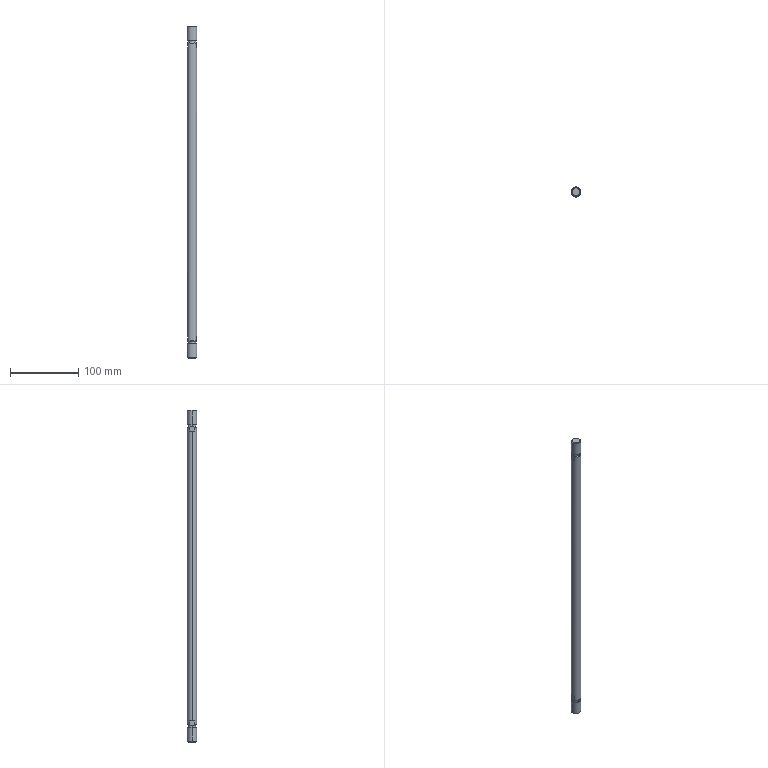Part | STEP file | rod_A_CDM2WB40_150_C76_0_ | 1 solid | 30 faces | box 14 x 14 x 488 mm | volume 74574 mm3 | plane 12 | cylinder 10 | cone 8 | commonest cylinder face diameters 14 x6 11.55 x4
STEP:
#1=CARTESIAN_POINT('',(5.775,0.,-454.));
#2=VERTEX_POINT('',#1);
#3=CARTESIAN_POINT('',(-5.775,0.,-454.));
#4=VERTEX_POINT('',#3);
#5=CARTESIAN_POINT('',(0.,0.,-454.));
#6=DIRECTION('',(0.,0.,1.));
#7=DIRECTION('',(1.,0.,0.));
#8=AXIS2_PLACEMENT_3D('',#5,#6,#7);
#9=CIRCLE('',#8,5.775);
#10=EDGE_CURVE('',#2,#4,#9,.T.);
#11=ORIENTED_EDGE('',*,*,#10,.T.);
#12=CARTESIAN_POINT('',(-7.,0.,-452.775));
#13=VERTEX_POINT('',#12);
#14=CARTESIAN_POINT('',(-5.775,0.,-454.));
#15=DIRECTION('',(-0.7071,0.,0.7071));
#16=VECTOR('',#15,1000.);
#17=LINE('',#14,#16);
#18=EDGE_CURVE('',#4,#13,#17,.T.);
#19=ORIENTED_EDGE('',*,*,#18,.T.);
#20=CARTESIAN_POINT('',(7.,0.,-452.775));
#21=VERTEX_POINT('',#20);
#22=CARTESIAN_POINT('',(0.,0.,-452.775));
#23=DIRECTION('',(0.,0.,1.));
#24=DIRECTION('',(1.,0.,0.));
#25=AXIS2_PLACEMENT_3D('',#22,#23,#24);
#26=CIRCLE('',#25,7.);
#27=EDGE_CURVE('',#21,#13,#26,.T.);
#28=ORIENTED_EDGE('',*,*,#27,.F.);
#29=CARTESIAN_POINT('',(5.775,0.,-454.));
#30=DIRECTION('',(0.7071,0.,0.7071));
#31=VECTOR('',#30,1000.);
#32=LINE('',#29,#31);
#33=EDGE_CURVE('',#2,#21,#32,.T.);
#34=ORIENTED_EDGE('',*,*,#33,.F.);
#35=EDGE_LOOP('',(#11,#19,#28,#34));
#36=FACE_OUTER_BOUND('',#35,.T.);
#37=CARTESIAN_POINT('',(0.,0.,-454.));
#38=DIRECTION('',(0.,0.,1.));
#39=DIRECTION('',(1.,0.,0.));
#40=AXIS2_PLACEMENT_3D('',#37,#38,#39);
#41=CONICAL_SURFACE('',#40,5.775,0.7854);
#42=ADVANCED_FACE('',(#36),#41,.T.);
#43=ORIENTED_EDGE('',*,*,#27,.T.);
#44=CARTESIAN_POINT('',(-7.,0.,-433.));
#45=VERTEX_POINT('',#44);
#46=CARTESIAN_POINT('',(-7.,0.,-454.));
#47=DIRECTION('',(0.,0.,1.));
#48=VECTOR('',#47,1000.);
#49=LINE('',#46,#48);
#50=EDGE_CURVE('',#13,#45,#49,.T.);
#51=ORIENTED_EDGE('',*,*,#50,.T.);
#52=CARTESIAN_POINT('',(7.,0.,-433.));
#53=VERTEX_POINT('',#52);
#54=CARTESIAN_POINT('',(0.,0.,-433.));
#55=DIRECTION('',(0.,0.,1.));
#56=DIRECTION('',(1.,0.,0.));
#57=AXIS2_PLACEMENT_3D('',#54,#55,#56);
#58=CIRCLE('',#57,7.);
#59=EDGE_CURVE('',#53,#45,#58,.T.);
#60=ORIENTED_EDGE('',*,*,#59,.F.);
#61=CARTESIAN_POINT('',(7.,0.,-454.));
#62=DIRECTION('',(0.,0.,1.));
#63=VECTOR('',#62,1000.);
#64=LINE('',#61,#63);
#65=EDGE_CURVE('',#21,#53,#64,.T.);
#66=ORIENTED_EDGE('',*,*,#65,.F.);
#67=EDGE_LOOP('',(#43,#51,#60,#66));
#68=FACE_OUTER_BOUND('',#67,.T.);
#69=CARTESIAN_POINT('',(0.,0.,-454.));
#70=DIRECTION('',(0.,0.,1.));
#71=DIRECTION('',(1.,0.,0.));
#72=AXIS2_PLACEMENT_3D('',#69,#70,#71);
#73=CYLINDRICAL_SURFACE('',#72,7.);
#74=ADVANCED_FACE('',(#68),#73,.T.);
#75=CARTESIAN_POINT('',(5.775,0.,-433.));
#76=VERTEX_POINT('',#75);
#77=CARTESIAN_POINT('',(-5.775,0.,-433.));
#78=VERTEX_POINT('',#77);
#79=CARTESIAN_POINT('',(0.,0.,-433.));
#80=DIRECTION('',(0.,0.,1.));
#81=DIRECTION('',(1.,0.,0.));
#82=AXIS2_PLACEMENT_3D('',#79,#80,#81);
#83=CIRCLE('',#82,5.775);
#84=EDGE_CURVE('',#76,#78,#83,.T.);
#85=ORIENTED_EDGE('',*,*,#84,.T.);
#86=CARTESIAN_POINT('',(-5.775,0.,-430.));
#87=VERTEX_POINT('',#86);
#88=CARTESIAN_POINT('',(-5.775,0.,-454.));
#89=DIRECTION('',(0.,0.,1.));
#90=VECTOR('',#89,1000.);
#91=LINE('',#88,#90);
#92=EDGE_CURVE('',#78,#87,#91,.T.);
#93=ORIENTED_EDGE('',*,*,#92,.T.);
#94=CARTESIAN_POINT('',(5.775,0.,-430.));
#95=VERTEX_POINT('',#94);
#96=CARTESIAN_POINT('',(0.,0.,-430.));
#97=DIRECTION('',(0.,0.,1.));
#98=DIRECTION('',(1.,0.,0.));
#99=AXIS2_PLACEMENT_3D('',#96,#97,#98);
#100=CIRCLE('',#99,5.775);
#101=EDGE_CURVE('',#95,#87,#100,.T.);
#102=ORIENTED_EDGE('',*,*,#101,.F.);
#103=CARTESIAN_POINT('',(5.775,0.,-454.));
#104=DIRECTION('',(0.,0.,1.));
#105=VECTOR('',#104,1000.);
#106=LINE('',#103,#105);
#107=EDGE_CURVE('',#76,#95,#106,.T.);
#108=ORIENTED_EDGE('',*,*,#107,.F.);
#109=EDGE_LOOP('',(#85,#93,#102,#108));
#110=FACE_OUTER_BOUND('',#109,.T.);
#111=CARTESIAN_POINT('',(0.,0.,-454.));
#112=DIRECTION('',(0.,0.,1.));
#113=DIRECTION('',(1.,0.,0.));
#114=AXIS2_PLACEMENT_3D('',#111,#112,#113);
#115=CYLINDRICAL_SURFACE('',#114,5.775);
#116=ADVANCED_FACE('',(#110),#115,.T.);
#117=ORIENTED_EDGE('',*,*,#101,.T.);
#118=CARTESIAN_POINT('',(-6.,0.,-429.775));
#119=VERTEX_POINT('',#118);
#120=CARTESIAN_POINT('',(-5.775,0.,-430.));
#121=DIRECTION('',(-0.7071,0.,0.7071));
#122=VECTOR('',#121,1000.);
#123=LINE('',#120,#122);
#124=EDGE_CURVE('',#87,#119,#123,.T.);
#125=ORIENTED_EDGE('',*,*,#124,.T.);
#126=CARTESIAN_POINT('',(-6.,3.606,-428.775));
#127=VERTEX_POINT('',#126);
#128=CARTESIAN_POINT('',(-6.,0.,-429.775));
#129=CARTESIAN_POINT('',(-6.,0.3144,-429.775));
#130=CARTESIAN_POINT('',(-6.,0.6332,-429.75));
#131=CARTESIAN_POINT('',(-6.,1.255,-429.653));
#132=CARTESIAN_POINT('',(-6.,1.561,-429.582));
#133=CARTESIAN_POINT('',(-6.,2.164,-429.403));
#134=CARTESIAN_POINT('',(-6.,2.462,-429.295));
#135=CARTESIAN_POINT('',(-6.,3.044,-429.052));
#136=CARTESIAN_POINT('',(-6.,3.328,-428.918));
#137=CARTESIAN_POINT('',(-6.,3.606,-428.775));
#138=B_SPLINE_CURVE_WITH_KNOTS('',3,(#128,#129,#130,#131,#132,#133,#134,#135,#136,#137),.UNSPECIFIED.,.F.,.F.,(4,2,2,2,4),(0.01366,0.0146,0.01554,0.01648,0.01742),.UNSPECIFIED.);
#139=EDGE_CURVE('',#119,#127,#138,.T.);
#140=ORIENTED_EDGE('',*,*,#139,.T.);
#141=CARTESIAN_POINT('',(6.,3.606,-428.775));
#142=VERTEX_POINT('',#141);
#143=CARTESIAN_POINT('',(0.,0.,-428.775));
#144=DIRECTION('',(0.,0.,1.));
#145=DIRECTION('',(1.,0.,0.));
#146=AXIS2_PLACEMENT_3D('',#143,#144,#145);
#147=CIRCLE('',#146,7.);
#148=EDGE_CURVE('',#142,#127,#147,.T.);
#149=ORIENTED_EDGE('',*,*,#148,.F.);
#150=CARTESIAN_POINT('',(6.,0.,-429.775));
#151=VERTEX_POINT('',#150);
#152=CARTESIAN_POINT('',(6.,3.606,-428.775));
#153=CARTESIAN_POINT('',(6.,3.328,-428.918));
#154=CARTESIAN_POINT('',(6.,3.044,-429.052));
#155=CARTESIAN_POINT('',(6.,2.462,-429.295));
#156=CARTESIAN_POINT('',(6.,2.164,-429.403));
#157=CARTESIAN_POINT('',(6.,1.561,-429.582));
#158=CARTESIAN_POINT('',(6.,1.255,-429.653));
#159=CARTESIAN_POINT('',(6.,0.6332,-429.75));
#160=CARTESIAN_POINT('',(6.,0.3144,-429.775));
#161=CARTESIAN_POINT('',(6.,0.,-429.775));
#162=B_SPLINE_CURVE_WITH_KNOTS('',3,(#152,#153,#154,#155,#156,#157,#158,#159,#160,#161),.UNSPECIFIED.,.F.,.F.,(4,2,2,2,4),(0.004778,0.005712,0.006646,0.00758,0.008514),.UNSPECIFIED.);
#163=EDGE_CURVE('',#142,#151,#162,.T.);
#164=ORIENTED_EDGE('',*,*,#163,.T.);
#165=CARTESIAN_POINT('',(5.775,0.,-430.));
#166=DIRECTION('',(0.7071,0.,0.7071));
#167=VECTOR('',#166,1000.);
#168=LINE('',#165,#167);
#169=EDGE_CURVE('',#95,#151,#168,.T.);
#170=ORIENTED_EDGE('',*,*,#169,.F.);
#171=EDGE_LOOP('',(#117,#125,#140,#149,#164,#170));
#172=FACE_OUTER_BOUND('',#171,.T.);
#173=CARTESIAN_POINT('',(0.,0.,-430.));
#174=DIRECTION('',(0.,0.,1.));
#175=DIRECTION('',(1.,0.,0.));
#176=AXIS2_PLACEMENT_3D('',#173,#174,#175);
#177=CONICAL_SURFACE('',#176,5.775,0.7854);
#178=ADVANCED_FACE('',(#172),#177,.T.);
#179=CARTESIAN_POINT('',(-6.,3.606,-423.));
#180=VERTEX_POINT('',#179);
#181=CARTESIAN_POINT('',(-7.,0.,-422.));
#182=VERTEX_POINT('',#181);
#183=CARTESIAN_POINT('',(-6.,3.606,-423.));
#184=CARTESIAN_POINT('',(-6.658,2.51,-422.342));
#185=CARTESIAN_POINT('',(-7.,1.278,-422.));
#186=CARTESIAN_POINT('',(-7.,0.,-422.));
#187=(BOUNDED_CURVE()B_SPLINE_CURVE(3,(#183,#184,#185,#186),.UNSPECIFIED.,.F.,.T.)B_SPLINE_CURVE_WITH_KNOTS((4,4),(5.742,6.283),.UNSPECIFIED.)CURVE()GEOMETRIC_REPRESENTATION_ITEM()RATIONAL_B_SPLINE_CURVE((1.,0.9757,0.9757,1.))REPRESENTATION_ITEM(''));
#188=EDGE_CURVE('',#180,#182,#187,.T.);
#189=ORIENTED_EDGE('',*,*,#188,.T.);
#190=CARTESIAN_POINT('',(-7.,0.,2.));
#191=VERTEX_POINT('',#190);
#192=CARTESIAN_POINT('',(-7.,0.,-454.));
#193=DIRECTION('',(0.,0.,1.));
#194=VECTOR('',#193,1000.);
#195=LINE('',#192,#194);
#196=EDGE_CURVE('',#182,#191,#195,.T.);
#197=ORIENTED_EDGE('',*,*,#196,.T.);
#198=CARTESIAN_POINT('',(-6.,3.606,3.));
#199=VERTEX_POINT('',#198);
#200=CARTESIAN_POINT('',(-7.,0.,2.));
#201=CARTESIAN_POINT('',(-7.,1.278,2.));
#202=CARTESIAN_POINT('',(-6.658,2.51,2.342));
#203=CARTESIAN_POINT('',(-6.,3.606,3.));
#204=(BOUNDED_CURVE()B_SPLINE_CURVE(3,(#200,#201,#202,#203),.UNSPECIFIED.,.F.,.T.)B_SPLINE_CURVE_WITH_KNOTS((4,4),(3.142,3.683),.UNSPECIFIED.)CURVE()GEOMETRIC_REPRESENTATION_ITEM()RATIONAL_B_SPLINE_CURVE((1.,0.9757,0.9757,1.))REPRESENTATION_ITEM(''));
#205=EDGE_CURVE('',#191,#199,#204,.T.);
#206=ORIENTED_EDGE('',*,*,#205,.T.);
#207=CARTESIAN_POINT('',(-6.,3.606,8.775));
#208=VERTEX_POINT('',#207);
#209=CARTESIAN_POINT('',(-6.,3.606,-454.));
#210=DIRECTION('',(0.,0.,1.));
#211=VECTOR('',#210,1000.);
#212=LINE('',#209,#211);
#213=EDGE_CURVE('',#199,#208,#212,.T.);
#214=ORIENTED_EDGE('',*,*,#213,.T.);
#215=CARTESIAN_POINT('',(6.,3.606,8.775));
#216=VERTEX_POINT('',#215);
#217=CARTESIAN_POINT('',(0.,0.,8.775));
#218=DIRECTION('',(0.,0.,1.));
#219=DIRECTION('',(1.,0.,0.));
#220=AXIS2_PLACEMENT_3D('',#217,#218,#219);
#221=CIRCLE('',#220,7.);
#222=EDGE_CURVE('',#216,#208,#221,.T.);
#223=ORIENTED_EDGE('',*,*,#222,.F.);
#224=CARTESIAN_POINT('',(6.,3.606,3.));
#225=VERTEX_POINT('',#224);
#226=CARTESIAN_POINT('',(6.,3.606,-454.));
#227=DIRECTION('',(0.,0.,-1.));
#228=VECTOR('',#227,1000.);
#229=LINE('',#226,#228);
#230=EDGE_CURVE('',#216,#225,#229,.T.);
#231=ORIENTED_EDGE('',*,*,#230,.T.);
#232=CARTESIAN_POINT('',(7.,0.,2.));
#233=VERTEX_POINT('',#232);
#234=CARTESIAN_POINT('',(6.,3.606,3.));
#235=CARTESIAN_POINT('',(6.658,2.51,2.342));
#236=CARTESIAN_POINT('',(7.,1.278,2.));
#237=CARTESIAN_POINT('',(7.,0.,2.));
#238=(BOUNDED_CURVE()B_SPLINE_CURVE(3,(#234,#235,#236,#237),.UNSPECIFIED.,.F.,.F.)B_SPLINE_CURVE_WITH_KNOTS((4,4),(2.6,3.142),.UNSPECIFIED.)CURVE()GEOMETRIC_REPRESENTATION_ITEM()RATIONAL_B_SPLINE_CURVE((1.,0.9757,0.9757,1.))REPRESENTATION_ITEM(''));
#239=EDGE_CURVE('',#225,#233,#238,.T.);
#240=ORIENTED_EDGE('',*,*,#239,.T.);
#241=CARTESIAN_POINT('',(7.,0.,-422.));
#242=VERTEX_POINT('',#241);
#243=CARTESIAN_POINT('',(7.,0.,-454.));
#244=DIRECTION('',(0.,0.,1.));
#245=VECTOR('',#244,1000.);
#246=LINE('',#243,#245);
#247=EDGE_CURVE('',#242,#233,#246,.T.);
#248=ORIENTED_EDGE('',*,*,#247,.F.);
#249=CARTESIAN_POINT('',(6.,3.606,-423.));
#250=VERTEX_POINT('',#249);
#251=CARTESIAN_POINT('',(7.,0.,-422.));
#252=CARTESIAN_POINT('',(7.,1.278,-422.));
#253=CARTESIAN_POINT('',(6.658,2.51,-422.342));
#254=CARTESIAN_POINT('',(6.,3.606,-423.));
#255=(BOUNDED_CURVE()B_SPLINE_CURVE(3,(#251,#252,#253,#254),.UNSPECIFIED.,.F.,.F.)B_SPLINE_CURVE_WITH_KNOTS((4,4),(0.,0.5411),.UNSPECIFIED.)CURVE()GEOMETRIC_REPRESENTATION_ITEM()RATIONAL_B_SPLINE_CURVE((1.,0.9757,0.9757,1.))REPRESENTATION_ITEM(''));
#256=EDGE_CURVE('',#242,#250,#255,.T.);
#257=ORIENTED_EDGE('',*,*,#256,.T.);
#258=CARTESIAN_POINT('',(6.,3.606,-454.));
#259=DIRECTION('',(0.,0.,-1.));
#260=VECTOR('',#259,1000.);
#261=LINE('',#258,#260);
#262=EDGE_CURVE('',#250,#142,#261,.T.);
#263=ORIENTED_EDGE('',*,*,#262,.T.);
#264=ORIENTED_EDGE('',*,*,#148,.T.);
#265=CARTESIAN_POINT('',(-6.,3.606,-454.));
#266=DIRECTION('',(0.,0.,1.));
#267=VECTOR('',#266,1000.);
#268=LINE('',#265,#267);
#269=EDGE_CURVE('',#127,#180,#268,.T.);
#270=ORIENTED_EDGE('',*,*,#269,.T.);
#271=EDGE_LOOP('',(#189,#197,#206,#214,#223,#231,#240,#248,#257,#263,#264,#270));
#272=FACE_OUTER_BOUND('',#271,.T.);
#273=CARTESIAN_POINT('',(0.,0.,-454.));
#274=DIRECTION('',(0.,0.,1.));
#275=DIRECTION('',(1.,0.,0.));
#276=AXIS2_PLACEMENT_3D('',#273,#274,#275);
#277=CYLINDRICAL_SURFACE('',#276,7.);
#278=ADVANCED_FACE('',(#272),#277,.T.);
#279=CARTESIAN_POINT('',(5.775,0.,10.));
#280=VERTEX_POINT('',#279);
#281=CARTESIAN_POINT('',(-5.775,0.,10.));
#282=VERTEX_POINT('',#281);
#283=CARTESIAN_POINT('',(0.,0.,10.));
#284=DIRECTION('',(0.,0.,1.));
#285=DIRECTION('',(1.,0.,0.));
#286=AXIS2_PLACEMENT_3D('',#283,#284,#285);
#287=CIRCLE('',#286,5.775);
#288=EDGE_CURVE('',#280,#282,#287,.T.);
#289=ORIENTED_EDGE('',*,*,#288,.F.);
#290=CARTESIAN_POINT('',(6.,0.,9.775));
#291=VERTEX_POINT('',#290);
#292=CARTESIAN_POINT('',(7.,0.,8.775));
#293=DIRECTION('',(0.7071,0.,-0.7071));
#294=VECTOR('',#293,1000.);
#295=LINE('',#292,#294);
#296=EDGE_CURVE('',#280,#291,#295,.T.);
#297=ORIENTED_EDGE('',*,*,#296,.T.);
#298=CARTESIAN_POINT('',(6.,0.,9.775));
#299=CARTESIAN_POINT('',(6.,0.3144,9.775));
#300=CARTESIAN_POINT('',(6.,0.6332,9.75));
#301=CARTESIAN_POINT('',(6.,1.255,9.653));
#302=CARTESIAN_POINT('',(6.,1.561,9.582));
#303=CARTESIAN_POINT('',(6.,2.164,9.403));
#304=CARTESIAN_POINT('',(6.,2.462,9.295));
#305=CARTESIAN_POINT('',(6.,3.044,9.052));
#306=CARTESIAN_POINT('',(6.,3.328,8.918));
#307=CARTESIAN_POINT('',(6.,3.606,8.775));
#308=B_SPLINE_CURVE_WITH_KNOTS('',3,(#298,#299,#300,#301,#302,#303,#304,#305,#306,#307),.UNSPECIFIED.,.F.,.F.,(4,2,2,2,4),(0.01366,0.0146,0.01554,0.01648,0.01742),.UNSPECIFIED.);
#309=EDGE_CURVE('',#291,#216,#308,.T.);
#310=ORIENTED_EDGE('',*,*,#309,.T.);
#311=ORIENTED_EDGE('',*,*,#222,.T.);
#312=CARTESIAN_POINT('',(-6.,0.,9.775));
#313=VERTEX_POINT('',#312);
#314=CARTESIAN_POINT('',(-6.,3.606,8.775));
#315=CARTESIAN_POINT('',(-6.,3.328,8.918));
#316=CARTESIAN_POINT('',(-6.,3.044,9.052));
#317=CARTESIAN_POINT('',(-6.,2.462,9.295));
#318=CARTESIAN_POINT('',(-6.,2.164,9.403));
#319=CARTESIAN_POINT('',(-6.,1.561,9.582));
#320=CARTESIAN_POINT('',(-6.,1.255,9.653));
#321=CARTESIAN_POINT('',(-6.,0.6332,9.75));
#322=CARTESIAN_POINT('',(-6.,0.3144,9.775));
#323=CARTESIAN_POINT('',(-6.,0.,9.775));
#324=B_SPLINE_CURVE_WITH_KNOTS('',3,(#314,#315,#316,#317,#318,#319,#320,#321,#322,#323),.UNSPECIFIED.,.F.,.F.,(4,2,2,2,4),(0.004778,0.005712,0.006646,0.00758,0.008514),.UNSPECIFIED.);
#325=EDGE_CURVE('',#208,#313,#324,.T.);
#326=ORIENTED_EDGE('',*,*,#325,.T.);
#327=CARTESIAN_POINT('',(-7.,0.,8.775));
#328=DIRECTION('',(-0.7071,0.,-0.7071));
#329=VECTOR('',#328,1000.);
#330=LINE('',#327,#329);
#331=EDGE_CURVE('',#282,#313,#330,.T.);
#332=ORIENTED_EDGE('',*,*,#331,.F.);
#333=EDGE_LOOP('',(#289,#297,#310,#311,#326,#332));
#334=FACE_OUTER_BOUND('',#333,.T.);
#335=CARTESIAN_POINT('',(0.,0.,8.775));
#336=DIRECTION('',(0.,0.,-1.));
#337=DIRECTION('',(-1.,0.,0.));
#338=AXIS2_PLACEMENT_3D('',#335,#336,#337);
#339=CONICAL_SURFACE('',#338,7.,0.7854);
#340=ADVANCED_FACE('',(#334),#339,.T.);
#341=ORIENTED_EDGE('',*,*,#288,.T.);
#342=CARTESIAN_POINT('',(-5.775,0.,13.));
#343=VERTEX_POINT('',#342);
#344=CARTESIAN_POINT('',(-5.775,0.,-454.));
#345=DIRECTION('',(0.,0.,1.));
#346=VECTOR('',#345,1000.);
#347=LINE('',#344,#346);
#348=EDGE_CURVE('',#282,#343,#347,.T.);
#349=ORIENTED_EDGE('',*,*,#348,.T.);
#350=CARTESIAN_POINT('',(5.775,0.,13.));
#351=VERTEX_POINT('',#350);
#352=CARTESIAN_POINT('',(0.,0.,13.));
#353=DIRECTION('',(0.,0.,1.));
#354=DIRECTION('',(1.,0.,0.));
#355=AXIS2_PLACEMENT_3D('',#352,#353,#354);
#356=CIRCLE('',#355,5.775);
#357=EDGE_CURVE('',#351,#343,#356,.T.);
#358=ORIENTED_EDGE('',*,*,#357,.F.);
#359=CARTESIAN_POINT('',(5.775,0.,-454.));
#360=DIRECTION('',(0.,0.,1.));
#361=VECTOR('',#360,1000.);
#362=LINE('',#359,#361);
#363=EDGE_CURVE('',#280,#351,#362,.T.);
#364=ORIENTED_EDGE('',*,*,#363,.F.);
#365=EDGE_LOOP('',(#341,#349,#358,#364));
#366=FACE_OUTER_BOUND('',#365,.T.);
#367=CARTESIAN_POINT('',(0.,0.,-454.));
#368=DIRECTION('',(0.,0.,1.));
#369=DIRECTION('',(1.,0.,0.));
#370=AXIS2_PLACEMENT_3D('',#367,#368,#369);
#371=CYLINDRICAL_SURFACE('',#370,5.775);
#372=ADVANCED_FACE('',(#366),#371,.T.);
#373=CARTESIAN_POINT('',(7.,0.,13.));
#374=VERTEX_POINT('',#373);
#375=CARTESIAN_POINT('',(-7.,0.,13.));
#376=VERTEX_POINT('',#375);
#377=CARTESIAN_POINT('',(0.,0.,13.));
#378=DIRECTION('',(0.,0.,1.));
#379=DIRECTION('',(1.,0.,0.));
#380=AXIS2_PLACEMENT_3D('',#377,#378,#379);
#381=CIRCLE('',#380,7.);
#382=EDGE_CURVE('',#374,#376,#381,.T.);
#383=ORIENTED_EDGE('',*,*,#382,.T.);
#384=CARTESIAN_POINT('',(-7.,0.,32.775));
#385=VERTEX_POINT('',#384);
#386=CARTESIAN_POINT('',(-7.,0.,-454.));
#387=DIRECTION('',(0.,0.,1.));
#388=VECTOR('',#387,1000.);
#389=LINE('',#386,#388);
#390=EDGE_CURVE('',#376,#385,#389,.T.);
#391=ORIENTED_EDGE('',*,*,#390,.T.);
#392=CARTESIAN_POINT('',(7.,0.,32.775));
#393=VERTEX_POINT('',#392);
#394=CARTESIAN_POINT('',(0.,0.,32.775));
#395=DIRECTION('',(0.,0.,1.));
#396=DIRECTION('',(1.,0.,0.));
#397=AXIS2_PLACEMENT_3D('',#394,#395,#396);
#398=CIRCLE('',#397,7.);
#399=EDGE_CURVE('',#393,#385,#398,.T.);
#400=ORIENTED_EDGE('',*,*,#399,.F.);
#401=CARTESIAN_POINT('',(7.,0.,-454.));
#402=DIRECTION('',(0.,0.,1.));
#403=VECTOR('',#402,1000.);
#404=LINE('',#401,#403);
#405=EDGE_CURVE('',#374,#393,#404,.T.);
#406=ORIENTED_EDGE('',*,*,#405,.F.);
#407=EDGE_LOOP('',(#383,#391,#400,#406));
#408=FACE_OUTER_BOUND('',#407,.T.);
#409=CARTESIAN_POINT('',(0.,0.,-454.));
#410=DIRECTION('',(0.,0.,1.));
#411=DIRECTION('',(1.,0.,0.));
#412=AXIS2_PLACEMENT_3D('',#409,#410,#411);
#413=CYLINDRICAL_SURFACE('',#412,7.);
#414=ADVANCED_FACE('',(#408),#413,.T.);
#415=CARTESIAN_POINT('',(5.775,0.,34.));
#416=VERTEX_POINT('',#415);
#417=CARTESIAN_POINT('',(-5.775,0.,34.));
#418=VERTEX_POINT('',#417);
#419=CARTESIAN_POINT('',(0.,0.,34.));
#420=DIRECTION('',(0.,0.,1.));
#421=DIRECTION('',(1.,0.,0.));
#422=AXIS2_PLACEMENT_3D('',#419,#420,#421);
#423=CIRCLE('',#422,5.775);
#424=EDGE_CURVE('',#416,#418,#423,.T.);
#425=ORIENTED_EDGE('',*,*,#424,.F.);
#426=CARTESIAN_POINT('',(7.,0.,32.775));
#427=DIRECTION('',(0.7071,0.,-0.7071));
#428=VECTOR('',#427,1000.);
#429=LINE('',#426,#428);
#430=EDGE_CURVE('',#416,#393,#429,.T.);
#431=ORIENTED_EDGE('',*,*,#430,.T.);
#432=ORIENTED_EDGE('',*,*,#399,.T.);
#433=CARTESIAN_POINT('',(-7.,0.,32.775));
#434=DIRECTION('',(-0.7071,0.,-0.7071));
#435=VECTOR('',#434,1000.);
#436=LINE('',#433,#435);
#437=EDGE_CURVE('',#418,#385,#436,.T.);
#438=ORIENTED_EDGE('',*,*,#437,.F.);
#439=EDGE_LOOP('',(#425,#431,#432,#438));
#440=FACE_OUTER_BOUND('',#439,.T.);
#441=CARTESIAN_POINT('',(0.,0.,32.775));
#442=DIRECTION('',(0.,0.,-1.));
#443=DIRECTION('',(-1.,0.,0.));
#444=AXIS2_PLACEMENT_3D('',#441,#442,#443);
#445=CONICAL_SURFACE('',#444,7.,0.7854);
#446=ADVANCED_FACE('',(#440),#445,.T.);
#447=CARTESIAN_POINT('',(0.,0.,34.));
#448=DIRECTION('',(0.,0.,1.));
#449=DIRECTION('',(1.,0.,0.));
#450=AXIS2_PLACEMENT_3D('',#447,#448,#449);
#451=CIRCLE('',#450,5.775);
#452=EDGE_CURVE('',#418,#416,#451,.T.);
#453=ORIENTED_EDGE('',*,*,#452,.T.);
#454=ORIENTED_EDGE('',*,*,#424,.T.);
#455=EDGE_LOOP('',(#453,#454));
#456=FACE_OUTER_BOUND('',#455,.T.);
#457=CARTESIAN_POINT('',(0.,0.,34.));
#458=DIRECTION('',(0.,0.,-1.));
#459=DIRECTION('',(-1.,0.,0.));
#460=AXIS2_PLACEMENT_3D('',#457,#458,#459);
#461=PLANE('',#460);
#462=ADVANCED_FACE('',(#456),#461,.F.);
#463=ORIENTED_EDGE('',*,*,#430,.F.);
#464=ORIENTED_EDGE('',*,*,#452,.F.);
#465=ORIENTED_EDGE('',*,*,#437,.T.);
#466=CARTESIAN_POINT('',(0.,0.,32.775));
#467=DIRECTION('',(0.,0.,1.));
#468=DIRECTION('',(1.,0.,0.));
#469=AXIS2_PLACEMENT_3D('',#466,#467,#468);
#470=CIRCLE('',#469,7.);
#471=EDGE_CURVE('',#385,#393,#470,.T.);
#472=ORIENTED_EDGE('',*,*,#471,.T.);
#473=EDGE_LOOP('',(#463,#464,#465,#472));
#474=FACE_OUTER_BOUND('',#473,.T.);
#475=CARTESIAN_POINT('',(0.,0.,32.775));
#476=DIRECTION('',(0.,0.,-1.));
#477=DIRECTION('',(-1.,0.,0.));
#478=AXIS2_PLACEMENT_3D('',#475,#476,#477);
#479=CONICAL_SURFACE('',#478,7.,0.7854);
#480=ADVANCED_FACE('',(#474),#479,.T.);
#481=ORIENTED_EDGE('',*,*,#390,.F.);
#482=CARTESIAN_POINT('',(0.,0.,13.));
#483=DIRECTION('',(0.,0.,1.));
#484=DIRECTION('',(1.,0.,0.));
#485=AXIS2_PLACEMENT_3D('',#482,#483,#484);
#486=CIRCLE('',#485,7.);
#487=EDGE_CURVE('',#376,#374,#486,.T.);
#488=ORIENTED_EDGE('',*,*,#487,.T.);
#489=ORIENTED_EDGE('',*,*,#405,.T.);
#490=ORIENTED_EDGE('',*,*,#471,.F.);
#491=EDGE_LOOP('',(#481,#488,#489,#490));
#492=FACE_OUTER_BOUND('',#491,.T.);
#493=CARTESIAN_POINT('',(0.,0.,-454.));
#494=DIRECTION('',(0.,0.,1.));
#495=DIRECTION('',(1.,0.,0.));
#496=AXIS2_PLACEMENT_3D('',#493,#494,#495);
#497=CYLINDRICAL_SURFACE('',#496,7.);
#498=ADVANCED_FACE('',(#492),#497,.T.);
#499=ORIENTED_EDGE('',*,*,#382,.F.);
#500=ORIENTED_EDGE('',*,*,#487,.F.);
#501=EDGE_LOOP('',(#499,#500));
#502=FACE_OUTER_BOUND('',#501,.T.);
#503=ORIENTED_EDGE('',*,*,#357,.T.);
#504=CARTESIAN_POINT('',(0.,0.,13.));
#505=DIRECTION('',(0.,0.,1.));
#506=DIRECTION('',(1.,0.,0.));
#507=AXIS2_PLACEMENT_3D('',#504,#505,#506);
#508=CIRCLE('',#507,5.775);
#509=EDGE_CURVE('',#343,#351,#508,.T.);
#510=ORIENTED_EDGE('',*,*,#509,.T.);
#511=EDGE_LOOP('',(#503,#510));
#512=FACE_BOUND('',#511,.T.);
#513=CARTESIAN_POINT('',(0.,7.,13.));
#514=DIRECTION('',(0.,0.,1.));
#515=DIRECTION('',(1.,0.,0.));
#516=AXIS2_PLACEMENT_3D('',#513,#514,#515);
#517=PLANE('',#516);
#518=ADVANCED_FACE('',(#502,#512),#517,.F.);
#519=ORIENTED_EDGE('',*,*,#348,.F.);
#520=CARTESIAN_POINT('',(0.,0.,10.));
#521=DIRECTION('',(0.,0.,1.));
#522=DIRECTION('',(1.,0.,0.));
#523=AXIS2_PLACEMENT_3D('',#520,#521,#522);
#524=CIRCLE('',#523,5.775);
#525=EDGE_CURVE('',#282,#280,#524,.T.);
#526=ORIENTED_EDGE('',*,*,#525,.T.);
#527=ORIENTED_EDGE('',*,*,#363,.T.);
#528=ORIENTED_EDGE('',*,*,#509,.F.);
#529=EDGE_LOOP('',(#519,#526,#527,#528));
#530=FACE_OUTER_BOUND('',#529,.T.);
#531=CARTESIAN_POINT('',(0.,0.,-454.));
#532=DIRECTION('',(0.,0.,1.));
#533=DIRECTION('',(1.,0.,0.));
#534=AXIS2_PLACEMENT_3D('',#531,#532,#533);
#535=CYLINDRICAL_SURFACE('',#534,5.775);
#536=ADVANCED_FACE('',(#530),#535,.T.);
#537=ORIENTED_EDGE('',*,*,#296,.F.);
#538=ORIENTED_EDGE('',*,*,#525,.F.);
#539=ORIENTED_EDGE('',*,*,#331,.T.);
#540=CARTESIAN_POINT('',(-6.,-3.606,8.775));
#541=VERTEX_POINT('',#540);
#542=CARTESIAN_POINT('',(-6.,0.,9.775));
#543=CARTESIAN_POINT('',(-6.,-0.3152,9.775));
#544=CARTESIAN_POINT('',(-6.,-0.628,9.75));
#545=CARTESIAN_POINT('',(-6.,-1.249,9.654));
#546=CARTESIAN_POINT('',(-6.,-1.559,9.582));
#547=CARTESIAN_POINT('',(-6.,-2.47,9.312));
#548=CARTESIAN_POINT('',(-6.,-3.047,9.063));
#549=CARTESIAN_POINT('',(-6.,-3.606,8.775));
#550=B_SPLINE_CURVE_WITH_KNOTS('',3,(#542,#543,#544,#545,#546,#547,#548,#549),.UNSPECIFIED.,.F.,.F.,(4,2,2,4),(0.008514,0.009451,0.01039,0.01226),.UNSPECIFIED.);
#551=EDGE_CURVE('',#313,#541,#550,.T.);
#552=ORIENTED_EDGE('',*,*,#551,.T.);
#553=CARTESIAN_POINT('',(6.,-3.606,8.775));
#554=VERTEX_POINT('',#553);
#555=CARTESIAN_POINT('',(0.,0.,8.775));
#556=DIRECTION('',(0.,0.,1.));
#557=DIRECTION('',(1.,0.,0.));
#558=AXIS2_PLACEMENT_3D('',#555,#556,#557);
#559=CIRCLE('',#558,7.);
#560=EDGE_CURVE('',#541,#554,#559,.T.);
#561=ORIENTED_EDGE('',*,*,#560,.T.);
#562=CARTESIAN_POINT('',(6.,-3.606,8.775));
#563=CARTESIAN_POINT('',(6.,-3.047,9.063));
#564=CARTESIAN_POINT('',(6.,-2.47,9.312));
#565=CARTESIAN_POINT('',(6.,-1.559,9.582));
#566=CARTESIAN_POINT('',(6.,-1.249,9.654));
#567=CARTESIAN_POINT('',(6.,-0.628,9.75));
#568=CARTESIAN_POINT('',(6.,-0.3152,9.775));
#569=CARTESIAN_POINT('',(6.,0.,9.775));
#570=B_SPLINE_CURVE_WITH_KNOTS('',3,(#562,#563,#564,#565,#566,#567,#568,#569),.UNSPECIFIED.,.F.,.F.,(4,2,2,4),(0.009896,0.01178,0.01272,0.01366),.UNSPECIFIED.);
#571=EDGE_CURVE('',#554,#291,#570,.T.);
#572=ORIENTED_EDGE('',*,*,#571,.T.);
#573=EDGE_LOOP('',(#537,#538,#539,#552,#561,#572));
#574=FACE_OUTER_BOUND('',#573,.T.);
#575=CARTESIAN_POINT('',(0.,0.,8.775));
#576=DIRECTION('',(0.,0.,-1.));
#577=DIRECTION('',(-1.,0.,0.));
#578=AXIS2_PLACEMENT_3D('',#575,#576,#577);
#579=CONICAL_SURFACE('',#578,7.,0.7854);
#580=ADVANCED_FACE('',(#574),#579,.T.);
#581=ORIENTED_EDGE('',*,*,#196,.F.);
#582=CARTESIAN_POINT('',(-6.,-3.606,-423.));
#583=VERTEX_POINT('',#582);
#584=CARTESIAN_POINT('',(-7.,0.,-422.));
#585=CARTESIAN_POINT('',(-7.,-1.278,-422.));
#586=CARTESIAN_POINT('',(-6.658,-2.51,-422.342));
#587=CARTESIAN_POINT('',(-6.,-3.606,-423.));
#588=(BOUNDED_CURVE()B_SPLINE_CURVE(3,(#584,#585,#586,#587),.UNSPECIFIED.,.F.,.F.)B_SPLINE_CURVE_WITH_KNOTS((4,4),(0.,0.5411),.UNSPECIFIED.)CURVE()GEOMETRIC_REPRESENTATION_ITEM()RATIONAL_B_SPLINE_CURVE((1.,0.9757,0.9757,1.))REPRESENTATION_ITEM(''));
#589=EDGE_CURVE('',#182,#583,#588,.T.);
#590=ORIENTED_EDGE('',*,*,#589,.T.);
#591=CARTESIAN_POINT('',(-6.,-3.606,-428.775));
#592=VERTEX_POINT('',#591);
#593=CARTESIAN_POINT('',(-6.,-3.606,-454.));
#594=DIRECTION('',(0.,0.,-1.));
#595=VECTOR('',#594,1000.);
#596=LINE('',#593,#595);
#597=EDGE_CURVE('',#583,#592,#596,.T.);
#598=ORIENTED_EDGE('',*,*,#597,.T.);
#599=CARTESIAN_POINT('',(6.,-3.606,-428.775));
#600=VERTEX_POINT('',#599);
#601=CARTESIAN_POINT('',(0.,0.,-428.775));
#602=DIRECTION('',(0.,0.,1.));
#603=DIRECTION('',(1.,0.,0.));
#604=AXIS2_PLACEMENT_3D('',#601,#602,#603);
#605=CIRCLE('',#604,7.);
#606=EDGE_CURVE('',#592,#600,#605,.T.);
#607=ORIENTED_EDGE('',*,*,#606,.T.);
#608=CARTESIAN_POINT('',(6.,-3.606,-423.));
#609=VERTEX_POINT('',#608);
#610=CARTESIAN_POINT('',(6.,-3.606,-454.));
#611=DIRECTION('',(0.,0.,1.));
#612=VECTOR('',#611,1000.);
#613=LINE('',#610,#612);
#614=EDGE_CURVE('',#600,#609,#613,.T.);
#615=ORIENTED_EDGE('',*,*,#614,.T.);
#616=CARTESIAN_POINT('',(6.,-3.606,-423.));
#617=CARTESIAN_POINT('',(6.658,-2.51,-422.342));
#618=CARTESIAN_POINT('',(7.,-1.278,-422.));
#619=CARTESIAN_POINT('',(7.,0.,-422.));
#620=(BOUNDED_CURVE()B_SPLINE_CURVE(3,(#616,#617,#618,#619),.UNSPECIFIED.,.F.,.T.)B_SPLINE_CURVE_WITH_KNOTS((4,4),(5.742,6.283),.UNSPECIFIED.)CURVE()GEOMETRIC_REPRESENTATION_ITEM()RATIONAL_B_SPLINE_CURVE((1.,0.9757,0.9757,1.))REPRESENTATION_ITEM(''));
#621=EDGE_CURVE('',#609,#242,#620,.T.);
#622=ORIENTED_EDGE('',*,*,#621,.T.);
#623=ORIENTED_EDGE('',*,*,#247,.T.);
#624=CARTESIAN_POINT('',(6.,-3.606,3.));
#625=VERTEX_POINT('',#624);
#626=CARTESIAN_POINT('',(7.,0.,2.));
#627=CARTESIAN_POINT('',(7.,-1.278,2.));
#628=CARTESIAN_POINT('',(6.658,-2.51,2.342));
#629=CARTESIAN_POINT('',(6.,-3.606,3.));
#630=(BOUNDED_CURVE()B_SPLINE_CURVE(3,(#626,#627,#628,#629),.UNSPECIFIED.,.F.,.T.)B_SPLINE_CURVE_WITH_KNOTS((4,4),(3.142,3.683),.UNSPECIFIED.)CURVE()GEOMETRIC_REPRESENTATION_ITEM()RATIONAL_B_SPLINE_CURVE((1.,0.9757,0.9757,1.))REPRESENTATION_ITEM(''));
#631=EDGE_CURVE('',#233,#625,#630,.T.);
#632=ORIENTED_EDGE('',*,*,#631,.T.);
#633=CARTESIAN_POINT('',(6.,-3.606,-454.));
#634=DIRECTION('',(0.,0.,1.));
#635=VECTOR('',#634,1000.);
#636=LINE('',#633,#635);
#637=EDGE_CURVE('',#625,#554,#636,.T.);
#638=ORIENTED_EDGE('',*,*,#637,.T.);
#639=ORIENTED_EDGE('',*,*,#560,.F.);
#640=CARTESIAN_POINT('',(-6.,-3.606,3.));
#641=VERTEX_POINT('',#640);
#642=CARTESIAN_POINT('',(-6.,-3.606,-454.));
#643=DIRECTION('',(0.,0.,-1.));
#644=VECTOR('',#643,1000.);
#645=LINE('',#642,#644);
#646=EDGE_CURVE('',#541,#641,#645,.T.);
#647=ORIENTED_EDGE('',*,*,#646,.T.);
#648=CARTESIAN_POINT('',(-6.,-3.606,3.));
#649=CARTESIAN_POINT('',(-6.658,-2.51,2.342));
#650=CARTESIAN_POINT('',(-7.,-1.278,2.));
#651=CARTESIAN_POINT('',(-7.,0.,2.));
#652=(BOUNDED_CURVE()B_SPLINE_CURVE(3,(#648,#649,#650,#651),.UNSPECIFIED.,.F.,.F.)B_SPLINE_CURVE_WITH_KNOTS((4,4),(2.6,3.142),.UNSPECIFIED.)CURVE()GEOMETRIC_REPRESENTATION_ITEM()RATIONAL_B_SPLINE_CURVE((1.,0.9757,0.9757,1.))REPRESENTATION_ITEM(''));
#653=EDGE_CURVE('',#641,#191,#652,.T.);
#654=ORIENTED_EDGE('',*,*,#653,.T.);
#655=EDGE_LOOP('',(#581,#590,#598,#607,#615,#622,#623,#632,#638,#639,#647,#654));
#656=FACE_OUTER_BOUND('',#655,.T.);
#657=CARTESIAN_POINT('',(0.,0.,-454.));
#658=DIRECTION('',(0.,0.,1.));
#659=DIRECTION('',(1.,0.,0.));
#660=AXIS2_PLACEMENT_3D('',#657,#658,#659);
#661=CYLINDRICAL_SURFACE('',#660,7.);
#662=ADVANCED_FACE('',(#656),#661,.T.);
#663=ORIENTED_EDGE('',*,*,#124,.F.);
#664=CARTESIAN_POINT('',(0.,0.,-430.));
#665=DIRECTION('',(0.,0.,1.));
#666=DIRECTION('',(1.,0.,0.));
#667=AXIS2_PLACEMENT_3D('',#664,#665,#666);
#668=CIRCLE('',#667,5.775);
#669=EDGE_CURVE('',#87,#95,#668,.T.);
#670=ORIENTED_EDGE('',*,*,#669,.T.);
#671=ORIENTED_EDGE('',*,*,#169,.T.);
#672=CARTESIAN_POINT('',(6.,0.,-429.775));
#673=CARTESIAN_POINT('',(6.,-0.3152,-429.775));
#674=CARTESIAN_POINT('',(6.,-0.628,-429.75));
#675=CARTESIAN_POINT('',(6.,-1.249,-429.654));
#676=CARTESIAN_POINT('',(6.,-1.559,-429.582));
#677=CARTESIAN_POINT('',(6.,-2.47,-429.312));
#678=CARTESIAN_POINT('',(6.,-3.047,-429.063));
#679=CARTESIAN_POINT('',(6.,-3.606,-428.775));
#680=B_SPLINE_CURVE_WITH_KNOTS('',3,(#672,#673,#674,#675,#676,#677,#678,#679),.UNSPECIFIED.,.F.,.F.,(4,2,2,4),(0.008514,0.009451,0.01039,0.01226),.UNSPECIFIED.);
#681=EDGE_CURVE('',#151,#600,#680,.T.);
#682=ORIENTED_EDGE('',*,*,#681,.T.);
#683=ORIENTED_EDGE('',*,*,#606,.F.);
#684=CARTESIAN_POINT('',(-6.,-3.606,-428.775));
#685=CARTESIAN_POINT('',(-6.,-3.047,-429.063));
#686=CARTESIAN_POINT('',(-6.,-2.47,-429.312));
#687=CARTESIAN_POINT('',(-6.,-1.559,-429.582));
#688=CARTESIAN_POINT('',(-6.,-1.249,-429.654));
#689=CARTESIAN_POINT('',(-6.,-0.628,-429.75));
#690=CARTESIAN_POINT('',(-6.,-0.3152,-429.775));
#691=CARTESIAN_POINT('',(-6.,0.,-429.775));
#692=B_SPLINE_CURVE_WITH_KNOTS('',3,(#684,#685,#686,#687,#688,#689,#690,#691),.UNSPECIFIED.,.F.,.F.,(4,2,2,4),(0.009896,0.01178,0.01272,0.01366),.UNSPECIFIED.);
#693=EDGE_CURVE('',#592,#119,#692,.T.);
#694=ORIENTED_EDGE('',*,*,#693,.T.);
#695=EDGE_LOOP('',(#663,#670,#671,#682,#683,#694));
#696=FACE_OUTER_BOUND('',#695,.T.);
#697=CARTESIAN_POINT('',(0.,0.,-430.));
#698=DIRECTION('',(0.,0.,1.));
#699=DIRECTION('',(1.,0.,0.));
#700=AXIS2_PLACEMENT_3D('',#697,#698,#699);
#701=CONICAL_SURFACE('',#700,5.775,0.7854);
#702=ADVANCED_FACE('',(#696),#701,.T.);
#703=ORIENTED_EDGE('',*,*,#92,.F.);
#704=CARTESIAN_POINT('',(0.,0.,-433.));
#705=DIRECTION('',(0.,0.,1.));
#706=DIRECTION('',(1.,0.,0.));
#707=AXIS2_PLACEMENT_3D('',#704,#705,#706);
#708=CIRCLE('',#707,5.775);
#709=EDGE_CURVE('',#78,#76,#708,.T.);
#710=ORIENTED_EDGE('',*,*,#709,.T.);
#711=ORIENTED_EDGE('',*,*,#107,.T.);
#712=ORIENTED_EDGE('',*,*,#669,.F.);
#713=EDGE_LOOP('',(#703,#710,#711,#712));
#714=FACE_OUTER_BOUND('',#713,.T.);
#715=CARTESIAN_POINT('',(0.,0.,-454.));
#716=DIRECTION('',(0.,0.,1.));
#717=DIRECTION('',(1.,0.,0.));
#718=AXIS2_PLACEMENT_3D('',#715,#716,#717);
#719=CYLINDRICAL_SURFACE('',#718,5.775);
#720=ADVANCED_FACE('',(#714),#719,.T.);
#721=ORIENTED_EDGE('',*,*,#84,.F.);
#722=ORIENTED_EDGE('',*,*,#709,.F.);
#723=EDGE_LOOP('',(#721,#722));
#724=FACE_BOUND('',#723,.T.);
#725=ORIENTED_EDGE('',*,*,#59,.T.);
#726=CARTESIAN_POINT('',(0.,0.,-433.));
#727=DIRECTION('',(0.,0.,1.));
#728=DIRECTION('',(1.,0.,0.));
#729=AXIS2_PLACEMENT_3D('',#726,#727,#728);
#730=CIRCLE('',#729,7.);
#731=EDGE_CURVE('',#45,#53,#730,.T.);
#732=ORIENTED_EDGE('',*,*,#731,.T.);
#733=EDGE_LOOP('',(#725,#732));
#734=FACE_OUTER_BOUND('',#733,.T.);
#735=CARTESIAN_POINT('',(0.,5.775,-433.));
#736=DIRECTION('',(0.,0.,-1.));
#737=DIRECTION('',(-1.,0.,0.));
#738=AXIS2_PLACEMENT_3D('',#735,#736,#737);
#739=PLANE('',#738);
#740=ADVANCED_FACE('',(#724,#734),#739,.F.);
#741=ORIENTED_EDGE('',*,*,#50,.F.);
#742=CARTESIAN_POINT('',(0.,0.,-452.775));
#743=DIRECTION('',(0.,0.,1.));
#744=DIRECTION('',(1.,0.,0.));
#745=AXIS2_PLACEMENT_3D('',#742,#743,#744);
#746=CIRCLE('',#745,7.);
#747=EDGE_CURVE('',#13,#21,#746,.T.);
#748=ORIENTED_EDGE('',*,*,#747,.T.);
#749=ORIENTED_EDGE('',*,*,#65,.T.);
#750=ORIENTED_EDGE('',*,*,#731,.F.);
#751=EDGE_LOOP('',(#741,#748,#749,#750));
#752=FACE_OUTER_BOUND('',#751,.T.);
#753=CARTESIAN_POINT('',(0.,0.,-454.));
#754=DIRECTION('',(0.,0.,1.));
#755=DIRECTION('',(1.,0.,0.));
#756=AXIS2_PLACEMENT_3D('',#753,#754,#755);
#757=CYLINDRICAL_SURFACE('',#756,7.);
#758=ADVANCED_FACE('',(#752),#757,.T.);
#759=ORIENTED_EDGE('',*,*,#18,.F.);
#760=CARTESIAN_POINT('',(0.,0.,-454.));
#761=DIRECTION('',(0.,0.,1.));
#762=DIRECTION('',(1.,0.,0.));
#763=AXIS2_PLACEMENT_3D('',#760,#761,#762);
#764=CIRCLE('',#763,5.775);
#765=EDGE_CURVE('',#4,#2,#764,.T.);
#766=ORIENTED_EDGE('',*,*,#765,.T.);
#767=ORIENTED_EDGE('',*,*,#33,.T.);
#768=ORIENTED_EDGE('',*,*,#747,.F.);
#769=EDGE_LOOP('',(#759,#766,#767,#768));
#770=FACE_OUTER_BOUND('',#769,.T.);
#771=CARTESIAN_POINT('',(0.,0.,-454.));
#772=DIRECTION('',(0.,0.,1.));
#773=DIRECTION('',(1.,0.,0.));
#774=AXIS2_PLACEMENT_3D('',#771,#772,#773);
#775=CONICAL_SURFACE('',#774,5.775,0.7854);
#776=ADVANCED_FACE('',(#770),#775,.T.);
#777=ORIENTED_EDGE('',*,*,#10,.F.);
#778=ORIENTED_EDGE('',*,*,#765,.F.);
#779=EDGE_LOOP('',(#777,#778));
#780=FACE_OUTER_BOUND('',#779,.T.);
#781=CARTESIAN_POINT('',(0.,5.775,-454.));
#782=DIRECTION('',(0.,0.,1.));
#783=DIRECTION('',(1.,0.,0.));
#784=AXIS2_PLACEMENT_3D('',#781,#782,#783);
#785=PLANE('',#784);
#786=ADVANCED_FACE('',(#780),#785,.F.);
#787=CARTESIAN_POINT('',(6.,-14.,3.));
#788=DIRECTION('',(0.,1.,0.));
#789=VECTOR('',#788,1000.);
#790=LINE('',#787,#789);
#791=EDGE_CURVE('',#625,#225,#790,.T.);
#792=ORIENTED_EDGE('',*,*,#791,.T.);
#793=ORIENTED_EDGE('',*,*,#230,.F.);
#794=ORIENTED_EDGE('',*,*,#309,.F.);
#795=ORIENTED_EDGE('',*,*,#571,.F.);
#796=ORIENTED_EDGE('',*,*,#637,.F.);
#797=EDGE_LOOP('',(#792,#793,#794,#795,#796));
#798=FACE_OUTER_BOUND('',#797,.T.);
#799=CARTESIAN_POINT('',(6.,-14.,3.));
#800=DIRECTION('',(-1.,0.,0.));
#801=DIRECTION('',(0.,0.,1.));
#802=AXIS2_PLACEMENT_3D('',#799,#800,#801);
#803=PLANE('',#802);
#804=ADVANCED_FACE('',(#798),#803,.F.);
#805=ORIENTED_EDGE('',*,*,#791,.F.);
#806=ORIENTED_EDGE('',*,*,#631,.F.);
#807=ORIENTED_EDGE('',*,*,#239,.F.);
#808=EDGE_LOOP('',(#805,#806,#807));
#809=FACE_OUTER_BOUND('',#808,.T.);
#810=CARTESIAN_POINT('',(7.,-14.,2.));
#811=DIRECTION('',(-0.7071,0.,-0.7071));
#812=DIRECTION('',(-0.7071,0.,0.7071));
#813=AXIS2_PLACEMENT_3D('',#810,#811,#812);
#814=PLANE('',#813);
#815=ADVANCED_FACE('',(#809),#814,.F.);
#816=CARTESIAN_POINT('',(-6.,-14.,3.));
#817=DIRECTION('',(0.,1.,0.));
#818=VECTOR('',#817,1000.);
#819=LINE('',#816,#818);
#820=EDGE_CURVE('',#641,#199,#819,.T.);
#821=ORIENTED_EDGE('',*,*,#820,.T.);
#822=ORIENTED_EDGE('',*,*,#205,.F.);
#823=ORIENTED_EDGE('',*,*,#653,.F.);
#824=EDGE_LOOP('',(#821,#822,#823));
#825=FACE_OUTER_BOUND('',#824,.T.);
#826=CARTESIAN_POINT('',(-6.,-14.,3.));
#827=DIRECTION('',(0.7071,0.,-0.7071));
#828=DIRECTION('',(-0.7071,0.,-0.7071));
#829=AXIS2_PLACEMENT_3D('',#826,#827,#828);
#830=PLANE('',#829);
#831=ADVANCED_FACE('',(#825),#830,.F.);
#832=ORIENTED_EDGE('',*,*,#820,.F.);
#833=ORIENTED_EDGE('',*,*,#646,.F.);
#834=ORIENTED_EDGE('',*,*,#551,.F.);
#835=ORIENTED_EDGE('',*,*,#325,.F.);
#836=ORIENTED_EDGE('',*,*,#213,.F.);
#837=EDGE_LOOP('',(#832,#833,#834,#835,#836));
#838=FACE_OUTER_BOUND('',#837,.T.);
#839=CARTESIAN_POINT('',(-6.,-14.,10.));
#840=DIRECTION('',(1.,0.,0.));
#841=DIRECTION('',(0.,0.,-1.));
#842=AXIS2_PLACEMENT_3D('',#839,#840,#841);
#843=PLANE('',#842);
#844=ADVANCED_FACE('',(#838),#843,.F.);
#845=ORIENTED_EDGE('',*,*,#621,.F.);
#846=CARTESIAN_POINT('',(6.,-14.,-423.));
#847=DIRECTION('',(0.,1.,0.));
#848=VECTOR('',#847,1000.);
#849=LINE('',#846,#848);
#850=EDGE_CURVE('',#609,#250,#849,.T.);
#851=ORIENTED_EDGE('',*,*,#850,.T.);
#852=ORIENTED_EDGE('',*,*,#256,.F.);
#853=EDGE_LOOP('',(#845,#851,#852));
#854=FACE_OUTER_BOUND('',#853,.T.);
#855=CARTESIAN_POINT('',(6.,-14.,-423.));
#856=DIRECTION('',(-0.7071,0.,0.7071));
#857=DIRECTION('',(0.7071,0.,0.7071));
#858=AXIS2_PLACEMENT_3D('',#855,#856,#857);
#859=PLANE('',#858);
#860=ADVANCED_FACE('',(#854),#859,.F.);
#861=ORIENTED_EDGE('',*,*,#163,.F.);
#862=ORIENTED_EDGE('',*,*,#262,.F.);
#863=ORIENTED_EDGE('',*,*,#850,.F.);
#864=ORIENTED_EDGE('',*,*,#614,.F.);
#865=ORIENTED_EDGE('',*,*,#681,.F.);
#866=EDGE_LOOP('',(#861,#862,#863,#864,#865));
#867=FACE_OUTER_BOUND('',#866,.T.);
#868=CARTESIAN_POINT('',(6.,-14.,-430.));
#869=DIRECTION('',(-1.,0.,0.));
#870=DIRECTION('',(0.,0.,1.));
#871=AXIS2_PLACEMENT_3D('',#868,#869,#870);
#872=PLANE('',#871);
#873=ADVANCED_FACE('',(#867),#872,.F.);
#874=ORIENTED_EDGE('',*,*,#188,.F.);
#875=CARTESIAN_POINT('',(-6.,-14.,-423.));
#876=DIRECTION('',(0.,1.,0.));
#877=VECTOR('',#876,1000.);
#878=LINE('',#875,#877);
#879=EDGE_CURVE('',#583,#180,#878,.T.);
#880=ORIENTED_EDGE('',*,*,#879,.F.);
#881=ORIENTED_EDGE('',*,*,#589,.F.);
#882=EDGE_LOOP('',(#874,#880,#881));
#883=FACE_OUTER_BOUND('',#882,.T.);
#884=CARTESIAN_POINT('',(-7.,-14.,-422.));
#885=DIRECTION('',(0.7071,0.,0.7071));
#886=DIRECTION('',(0.7071,0.,-0.7071));
#887=AXIS2_PLACEMENT_3D('',#884,#885,#886);
#888=PLANE('',#887);
#889=ADVANCED_FACE('',(#883),#888,.F.);
#890=ORIENTED_EDGE('',*,*,#693,.F.);
#891=ORIENTED_EDGE('',*,*,#597,.F.);
#892=ORIENTED_EDGE('',*,*,#879,.T.);
#893=ORIENTED_EDGE('',*,*,#269,.F.);
#894=ORIENTED_EDGE('',*,*,#139,.F.);
#895=EDGE_LOOP('',(#890,#891,#892,#893,#894));
#896=FACE_OUTER_BOUND('',#895,.T.);
#897=CARTESIAN_POINT('',(-6.,-14.,-423.));
#898=DIRECTION('',(1.,0.,0.));
#899=DIRECTION('',(0.,0.,-1.));
#900=AXIS2_PLACEMENT_3D('',#897,#898,#899);
#901=PLANE('',#900);
#902=ADVANCED_FACE('',(#896),#901,.F.);
#903=CLOSED_SHELL('',(#42,#74,#116,#178,#278,#340,#372,#414,#446,#462,#480,#498,#518,#536,#580,#662,#702,#720,#740,#758,#776,#786,#804,#815,#831,#844,#860,#873,#889,#902));
#904=MANIFOLD_SOLID_BREP('',#903);
#905=CARTESIAN_POINT('',(0.,0.,0.));
#906=DIRECTION('',(0.,0.,1.));
#907=DIRECTION('',(1.,0.,0.));
#908=AXIS2_PLACEMENT_3D('',#905,#906,#907);
#909=(LENGTH_UNIT()NAMED_UNIT(*)SI_UNIT(.MILLI.,.METRE.));
#910=UNCERTAINTY_MEASURE_WITH_UNIT(LENGTH_MEASURE(0.00001),#909,'','');
#911=(NAMED_UNIT(*)PLANE_ANGLE_UNIT()SI_UNIT($,.RADIAN.));
#912=(NAMED_UNIT(*)SI_UNIT($,.STERADIAN.)SOLID_ANGLE_UNIT());
#913=(GEOMETRIC_REPRESENTATION_CONTEXT(3)GLOBAL_UNCERTAINTY_ASSIGNED_CONTEXT((#910))GLOBAL_UNIT_ASSIGNED_CONTEXT((#909,#911,#912))REPRESENTATION_CONTEXT('',''));
#914=ADVANCED_BREP_SHAPE_REPRESENTATION('',(#904,#908),#913);